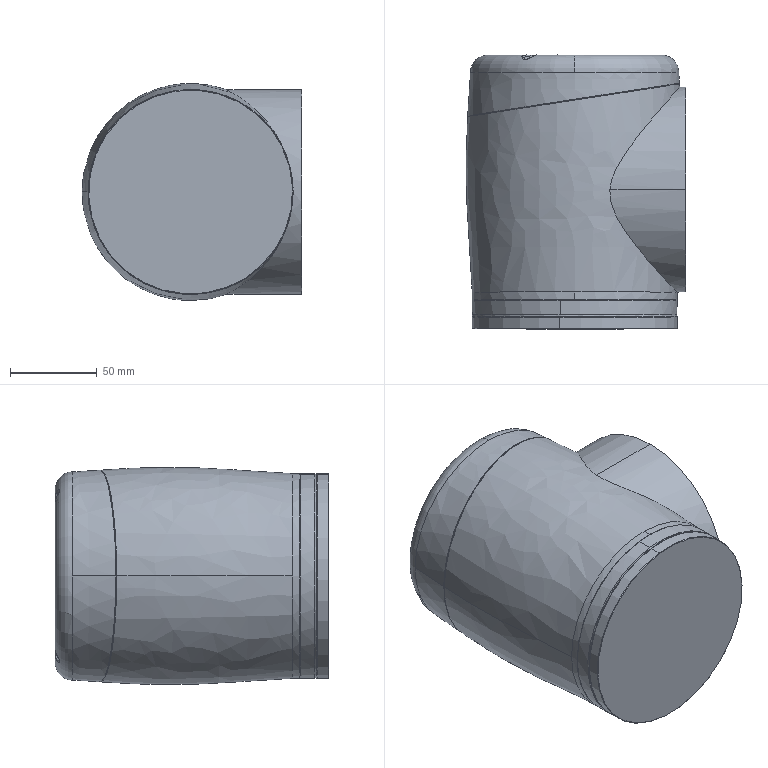Part | SolidWorks | features BaseBody 1 | 1 solid | 100 faces | box 126.523 x 157.65 x 125.047 mm | volume 1928290 mm3 | plane 54 | spline 19 | cylinder 19 | cone 4 | torus 4 | commonest cylinder face diameters 118 x12 6.2 x6 3.5 x1